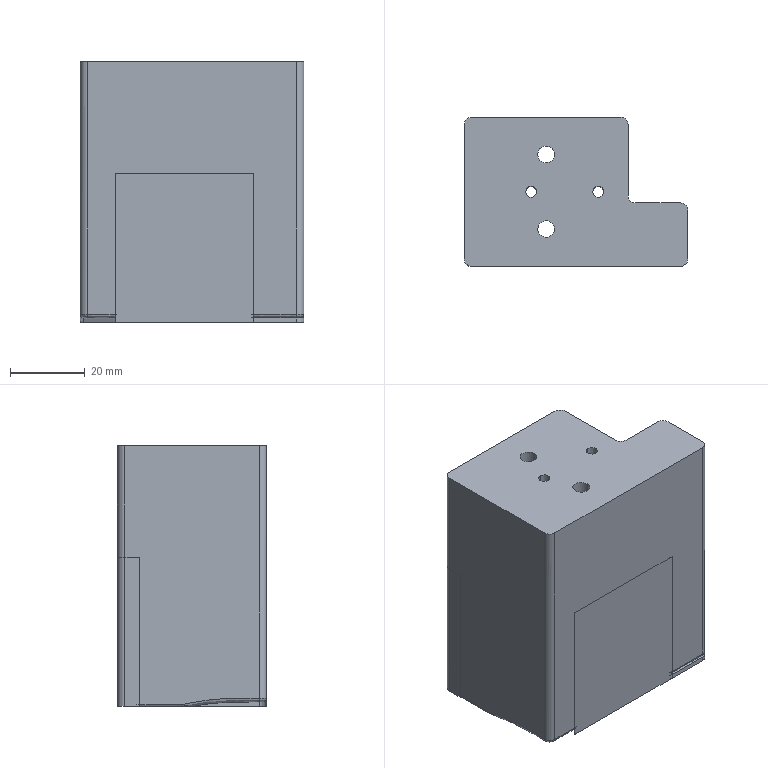NC program | NX | posted with a generic post | part box 60.004 x 40.015 x 70 mm
Lines 4494 to 4654 of 35085:
(FLOOR_WALL_1_COPY_COPY , TOOL : D10JING)
N8986 T10 M6
N8988 G54
N8990 G17 G0 G90 X20.288 Y-3.5 B0. C0. S9500 M3
N8992 G43 Z30. H10
N8994 Z-18.5
N8996 G94 G1 Z-20. F1000.
N8998 X19.827 Y-2.544
N9000 G3 X19. Y-1.981 R1.
N9002 G2 X12.702 Y3.411 R7.
N9004 G1 X9.671 Y16.411
N9006 G2 X15.841 Y24.97 R7.
N9008 G3 X16.657 Y25.548 R1.
N9010 G1 X17.095 Y26.5
N9012 Z-18.5
N9014 G0 Z30.
N9016 X-21.245
N9018 Z-18.5
N9020 G1 Z-20.
N9022 X-20.807 Y25.548
N9024 G3 X-19.991 Y24.97 R1.
N9026 G2 X-13.639 Y18. R7.
N9028 G1 Y-9.359
N9030 G2 X-15.213 Y-14.744 R10.
N9032 X-20.146 Y-19.781 R16.728
N9034 X-28.073 Y-21.166 R10.
N9036 G1 X-28.965 Y-20.947
N9038 X-29.665 Y-20.775
N9040 G2 X-34.97 Y-14.623 R7.
N9042 G3 X-35.548 Y-13.807 R1.
N9044 G1 X-36.5 Y-13.37
N9046 Z-18.5
N9048 G0 Z30.
N9050 X-21.245 Y26.5
N9052 Z-38.5
N9054 G1 Z-40.
N9056 X-20.807 Y25.548
N9058 G3 X-19.991 Y24.97 R1.
N9060 G2 X-13.639 Y18. R7.
N9062 G1 Y-9.359
N9064 G2 X-15.213 Y-14.744 R10.
N9066 X-20.146 Y-19.781 R16.728
N9068 X-28.073 Y-21.166 R10.
N9070 G1 X-28.965 Y-20.947
N9072 X-29.665 Y-20.775
N9074 G2 X-34.97 Y-14.623 R7.
N9076 G3 X-35.548 Y-13.807 R1.
N9078 G1 X-36.5 Y-13.37
N9080 Z-38.5
N9082 G0 Z30.
N9084 X20.288 Y-3.5
N9086 Z-38.5
N9088 G1 Z-40.
N9090 X19.827 Y-2.544
N9092 G3 X19. Y-1.981 R1.
N9094 G2 X12.702 Y3.411 R7.
N9096 G1 X9.671 Y16.411
N9098 G2 X15.841 Y24.97 R7.
N9100 G3 X16.657 Y25.548 R1.
N9102 G1 X17.095 Y26.5
N9104 Z-38.5
N9106 G0 Z30.
(FLOOR_WALL_1_COPY , TOOL : D10JING)
N9108 X-21.174 Y-26.5
N9110 Z-38.5
N9112 G1 Z-40.
N9114 X-20.076 Y-25.866
N9116 G3 X-19.576 Y-25. R1.
N9118 G1 Y-20.
N9120 G3 X-14.791 Y-15.012 R17.228
N9122 X-14.647 Y-14.781 R10.5
N9124 G1 Y-25.
N9126 G2 X-15.147 Y-25.866 R1.
N9128 G1 X-16.245 Y-26.5
N9130 Z-38.5
N9132 G0 Z30.
N9134 Y26.5
N9136 Z-38.5
N9138 G1 Z-40.
N9140 X-15.147 Y25.866
N9142 G2 X-14.647 Y25. R1.
N9144 G1 Y22.511
N9146 Z-38.5
N9148 G0 Z30.
N9150 X-11.316 Y-26.5
N9152 Z-38.5
N9154 G1 Z-40.
N9156 X-10.217 Y-25.866
N9158 G3 X-9.717 Y-25. R1.
N9160 G1 Y25.
N9162 X-4.788
N9164 Y-25.
N9166 X0.141
N9168 Y25.
N9170 X5.071
N9172 Y-25.
N9174 X10.
N9176 Y12.798
N9178 X12.215 Y3.297
N9180 G3 X14.929 Y-0.932 R7.5
N9182 G1 Y-24.358
N9184 G2 X14.429 Y-25.224 R1.
N9186 G1 X12.224 Y-26.497
N9188 Z-38.5
N9190 G0 Z30.
N9192 X10. Y12.798
N9194 Z-38.5
N9196 G1 Z-40.
N9198 X9.184 Y16.297
N9200 G2 X10. Y21.762 R7.5
N9202 G1 Y25.
N9204 G3 X9.5 Y25.866 R1.
N9206 G1 X8.402 Y26.5
N9208 Z-38.5
N9210 G0 Z30.
N9212 X20.5 Y-3.94
N9214 Z-38.5
N9216 G1 Z-40.
N9218 X19.827 Y-2.544
N9220 G3 X19. Y-1.981 R1.
N9222 G2 X12.702 Y3.411 R7.
N9224 G1 X9.671 Y16.411
N9226 G2 X15.841 Y24.97 R7.
N9228 G3 X16.657 Y25.548 R1.
N9230 G1 X17.095 Y26.5
N9232 Z-38.5
N9234 G0 Z30.
N9236 X-21.245
N9238 Z-38.5
N9240 G1 Z-40.
N9242 X-20.807 Y25.548
N9244 G3 X-19.991 Y24.97 R1.
N9246 G2 X-13.639 Y18. R7.
N9248 G1 Y-9.359
N9250 G2 X-15.213 Y-14.744 R10.
N9252 X-20.146 Y-19.781 R16.728
N9254 X-28.073 Y-21.166 R10.
N9256 G1 X-28.965 Y-20.947
N9258 X-29.665 Y-20.775
N9260 G2 X-34.97 Y-14.623 R7.
N9262 G3 X-35.548 Y-13.807 R1.
N9264 G1 X-36.5 Y-13.37
N9266 Z-38.5
N9268 G0 Z30.
N9270 M5
(DRILLING_COPY_COPY_COPY_COPY_COPY_COPY_COPY , TOOL : D8)
N9272 T07 M6
N9274 G54
N9276 G17 G0 G90 X-8. Y10. B0. C0. S1500 M3
N9278 G43 Z30. H7
N9280 G94 G83 G98 Z-55. F180. Q2. R-37.
N9282 Y-10.
N9284 G80
N9286 G0 X-8. Y-10. Z30.
N9288 M5